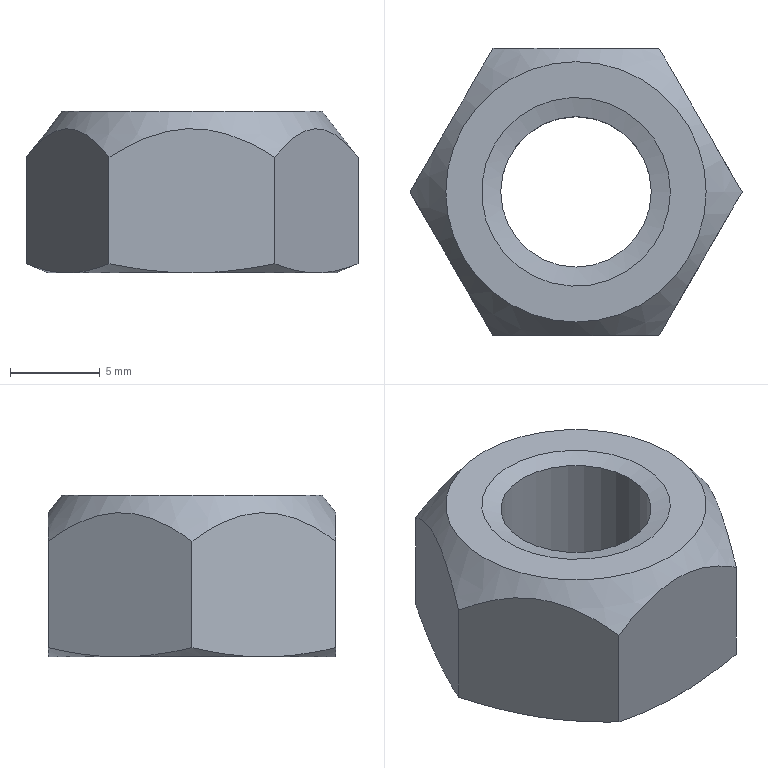Part | STEP file | Screw_set_M10x45 | 1 solid | 19 faces | box 18.475 x 16 x 9 mm | volume 1440 mm3 | cone 10 | plane 8 | cylinder 1 | commonest cylinder face diameters 8.376 x1